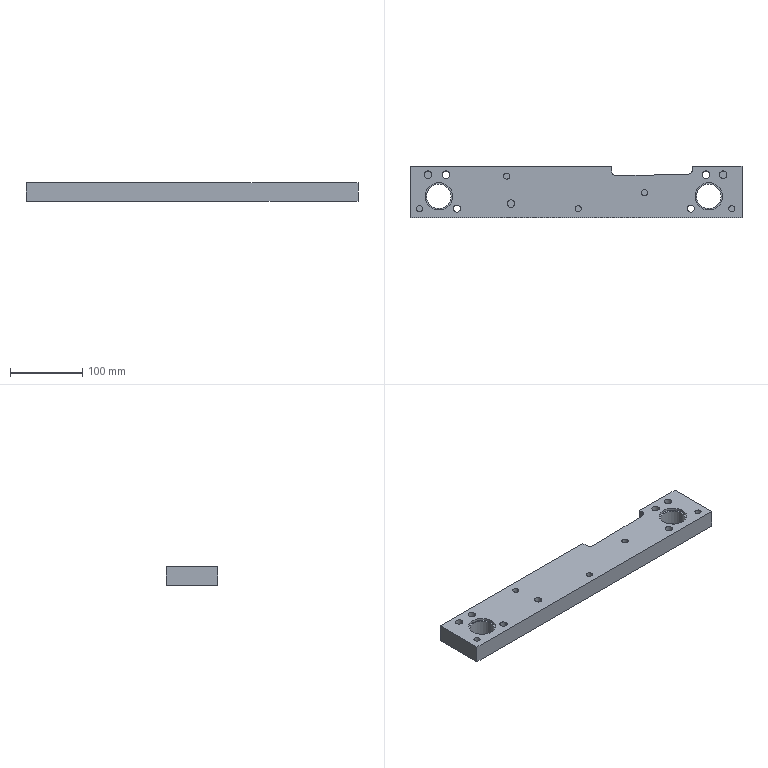Part | NX | features LIN_SOLID_COLOR 2 | 1 solid | 54 faces | box 460 x 72 x 25 mm | volume 695403 mm3 | plane 30 | cylinder 24 | commonest cylinder face diameters 8.5 x5 10.3 x5 10 x4 10.001 x2 10.31 x2 14 x2
STEP:
#1=CARTESIAN_POINT('',(747.152,-157.,0.));
#2=VERTEX_POINT('',#1);
#3=CARTESIAN_POINT('',(741.997,-157.,0.));
#4=DIRECTION('',(0.,0.,1.));
#5=DIRECTION('',(1.,0.,0.));
#6=AXIS2_PLACEMENT_3D('',#3,#4,#5);
#7=CIRCLE('',#6,5.155);
#8=EDGE_CURVE('',#2,#2,#7,.T.);
#9=ORIENTED_EDGE('',*,*,#8,.T.);
#10=EDGE_LOOP('',(#9));
#11=FACE_BOUND('',#10,.T.);
#12=CARTESIAN_POINT('',(423.158,-157.,0.));
#13=VERTEX_POINT('',#12);
#14=CARTESIAN_POINT('',(418.003,-157.,0.));
#15=DIRECTION('',(0.,0.,1.));
#16=DIRECTION('',(1.,0.,0.));
#17=AXIS2_PLACEMENT_3D('',#14,#15,#16);
#18=CIRCLE('',#17,5.155);
#19=EDGE_CURVE('',#13,#13,#18,.T.);
#20=ORIENTED_EDGE('',*,*,#19,.T.);
#21=EDGE_LOOP('',(#20));
#22=FACE_BOUND('',#21,.T.);
#23=CARTESIAN_POINT('',(750.,-140.,0.));
#24=VERTEX_POINT('',#23);
#25=CARTESIAN_POINT('',(767.,-140.,0.));
#26=DIRECTION('',(0.,0.,-1.));
#27=DIRECTION('',(-1.,0.,0.));
#28=AXIS2_PLACEMENT_3D('',#25,#26,#27);
#29=CIRCLE('',#28,17.);
#30=EDGE_CURVE('',#24,#24,#29,.T.);
#31=ORIENTED_EDGE('',*,*,#30,.F.);
#32=EDGE_LOOP('',(#31));
#33=FACE_BOUND('',#32,.T.);
#34=CARTESIAN_POINT('',(376.,-140.,0.));
#35=VERTEX_POINT('',#34);
#36=CARTESIAN_POINT('',(393.,-140.,0.));
#37=DIRECTION('',(0.,0.,-1.));
#38=DIRECTION('',(-1.,0.,0.));
#39=AXIS2_PLACEMENT_3D('',#36,#37,#38);
#40=CIRCLE('',#39,17.);
#41=EDGE_CURVE('',#35,#35,#40,.T.);
#42=ORIENTED_EDGE('',*,*,#41,.F.);
#43=EDGE_LOOP('',(#42));
#44=FACE_BOUND('',#43,.T.);
#45=CARTESIAN_POINT('',(757.85,-110.,0.));
#46=VERTEX_POINT('',#45);
#47=CARTESIAN_POINT('',(763.,-110.,0.));
#48=DIRECTION('',(0.,0.,-1.));
#49=DIRECTION('',(-1.,0.,0.));
#50=AXIS2_PLACEMENT_3D('',#47,#48,#49);
#51=CIRCLE('',#50,5.15);
#52=EDGE_CURVE('',#46,#46,#51,.T.);
#53=ORIENTED_EDGE('',*,*,#52,.F.);
#54=EDGE_LOOP('',(#53));
#55=FACE_BOUND('',#54,.T.);
#56=CARTESIAN_POINT('',(397.85,-110.,0.));
#57=VERTEX_POINT('',#56);
#58=CARTESIAN_POINT('',(403.,-110.,0.));
#59=DIRECTION('',(0.,0.,-1.));
#60=DIRECTION('',(-1.,0.,0.));
#61=AXIS2_PLACEMENT_3D('',#58,#59,#60);
#62=CIRCLE('',#61,5.15);
#63=EDGE_CURVE('',#57,#57,#62,.T.);
#64=ORIENTED_EDGE('',*,*,#63,.F.);
#65=EDGE_LOOP('',(#64));
#66=FACE_BOUND('',#65,.T.);
#67=CARTESIAN_POINT('',(646.028,-130.524,0.));
#68=VERTEX_POINT('',#67);
#69=CARTESIAN_POINT('',(638.826,-123.653,0.));
#70=VERTEX_POINT('',#69);
#71=CARTESIAN_POINT('',(642.098,-127.434,0.));
#72=DIRECTION('',(0.,0.,-1.));
#73=DIRECTION('',(-1.,0.,0.));
#74=AXIS2_PLACEMENT_3D('',#71,#72,#73);
#75=CIRCLE('',#74,5.);
#76=EDGE_CURVE('',#68,#70,#75,.T.);
#77=ORIENTED_EDGE('',*,*,#76,.F.);
#78=CARTESIAN_POINT('',(731.927,-128.503,0.));
#79=VERTEX_POINT('',#78);
#80=CARTESIAN_POINT('',(745.016,-128.195,0.));
#81=DIRECTION('',(-0.9997,-0.02352,0.));
#82=VECTOR('',#81,1000.);
#83=LINE('',#80,#82);
#84=EDGE_CURVE('',#79,#68,#83,.T.);
#85=ORIENTED_EDGE('',*,*,#84,.F.);
#86=CARTESIAN_POINT('',(738.798,-121.301,0.));
#87=VERTEX_POINT('',#86);
#88=CARTESIAN_POINT('',(735.708,-125.231,0.));
#89=DIRECTION('',(0.,0.,-1.));
#90=DIRECTION('',(-1.,0.,0.));
#91=AXIS2_PLACEMENT_3D('',#88,#89,#90);
#92=CIRCLE('',#91,5.);
#93=EDGE_CURVE('',#87,#79,#92,.T.);
#94=ORIENTED_EDGE('',*,*,#93,.F.);
#95=CARTESIAN_POINT('',(738.515,-109.271,0.));
#96=VERTEX_POINT('',#95);
#97=CARTESIAN_POINT('',(735.947,-0.1424,0.));
#98=DIRECTION('',(0.02352,-0.9997,0.));
#99=VECTOR('',#98,1000.);
#100=LINE('',#97,#99);
#101=EDGE_CURVE('',#96,#87,#100,.T.);
#102=ORIENTED_EDGE('',*,*,#101,.F.);
#103=CARTESIAN_POINT('',(744.35,-102.204,0.));
#104=VERTEX_POINT('',#103);
#105=CARTESIAN_POINT('',(737.352,-102.368,0.));
#106=DIRECTION('',(0.,0.,-1.));
#107=DIRECTION('',(-1.,0.,0.));
#108=AXIS2_PLACEMENT_3D('',#105,#106,#107);
#109=CIRCLE('',#108,7.);
#110=EDGE_CURVE('',#104,#96,#109,.T.);
#111=ORIENTED_EDGE('',*,*,#110,.F.);
#112=CARTESIAN_POINT('',(744.251,-98.,0.));
#113=VERTEX_POINT('',#112);
#114=CARTESIAN_POINT('',(741.946,-0.001282,0.));
#115=DIRECTION('',(-0.02352,0.9997,0.));
#116=VECTOR('',#115,1000.);
#117=LINE('',#114,#116);
#118=EDGE_CURVE('',#113,#104,#117,.F.);
#119=ORIENTED_EDGE('',*,*,#118,.F.);
#120=CARTESIAN_POINT('',(813.,-98.,0.));
#121=VERTEX_POINT('',#120);
#122=CARTESIAN_POINT('',(742.,-98.,0.));
#123=DIRECTION('',(1.,0.,0.));
#124=VECTOR('',#123,1000.);
#125=LINE('',#122,#124);
#126=EDGE_CURVE('',#113,#121,#125,.T.);
#127=ORIENTED_EDGE('',*,*,#126,.T.);
#128=CARTESIAN_POINT('',(813.,-170.,0.));
#129=VERTEX_POINT('',#128);
#130=CARTESIAN_POINT('',(813.,0.,0.));
#131=DIRECTION('',(0.,-1.,0.));
#132=VECTOR('',#131,1000.);
#133=LINE('',#130,#132);
#134=EDGE_CURVE('',#121,#129,#133,.T.);
#135=ORIENTED_EDGE('',*,*,#134,.T.);
#136=CARTESIAN_POINT('',(353.,-170.,0.));
#137=VERTEX_POINT('',#136);
#138=CARTESIAN_POINT('',(788.,-170.,0.));
#139=DIRECTION('',(1.,0.,0.));
#140=VECTOR('',#139,1000.);
#141=LINE('',#138,#140);
#142=EDGE_CURVE('',#137,#129,#141,.T.);
#143=ORIENTED_EDGE('',*,*,#142,.F.);
#144=CARTESIAN_POINT('',(353.,-98.,0.));
#145=VERTEX_POINT('',#144);
#146=CARTESIAN_POINT('',(353.,0.,0.));
#147=DIRECTION('',(0.,-1.,0.));
#148=VECTOR('',#147,1000.);
#149=LINE('',#146,#148);
#150=EDGE_CURVE('',#145,#137,#149,.T.);
#151=ORIENTED_EDGE('',*,*,#150,.F.);
#152=CARTESIAN_POINT('',(529.5,-98.,0.));
#153=VERTEX_POINT('',#152);
#154=CARTESIAN_POINT('',(742.,-98.,0.));
#155=DIRECTION('',(1.,0.,0.));
#156=VECTOR('',#155,1000.);
#157=LINE('',#154,#156);
#158=EDGE_CURVE('',#145,#153,#157,.T.);
#159=ORIENTED_EDGE('',*,*,#158,.T.);
#160=CARTESIAN_POINT('',(529.5,-111.161,0.));
#161=VERTEX_POINT('',#160);
#162=CARTESIAN_POINT('',(529.5,0.,0.));
#163=DIRECTION('',(0.,1.,0.));
#164=VECTOR('',#163,1000.);
#165=LINE('',#162,#164);
#166=EDGE_CURVE('',#161,#153,#165,.T.);
#167=ORIENTED_EDGE('',*,*,#166,.F.);
#168=CARTESIAN_POINT('',(536.539,-118.2,0.));
#169=VERTEX_POINT('',#168);
#170=CARTESIAN_POINT('',(532.682,-115.018,0.));
#171=DIRECTION('',(0.,0.,-1.));
#172=DIRECTION('',(-1.,0.,0.));
#173=AXIS2_PLACEMENT_3D('',#170,#171,#172);
#174=CIRCLE('',#173,5.);
#175=EDGE_CURVE('',#169,#161,#174,.T.);
#176=ORIENTED_EDGE('',*,*,#175,.F.);
#177=CARTESIAN_POINT('',(588.461,-118.2,0.));
#178=VERTEX_POINT('',#177);
#179=CARTESIAN_POINT('',(742.,-118.2,0.));
#180=DIRECTION('',(-1.,0.,0.));
#181=VECTOR('',#180,1000.);
#182=LINE('',#179,#181);
#183=EDGE_CURVE('',#178,#169,#182,.T.);
#184=ORIENTED_EDGE('',*,*,#183,.F.);
#185=CARTESIAN_POINT('',(595.5,-111.161,0.));
#186=VERTEX_POINT('',#185);
#187=CARTESIAN_POINT('',(592.318,-115.018,0.));
#188=DIRECTION('',(0.,0.,-1.));
#189=DIRECTION('',(-1.,0.,0.));
#190=AXIS2_PLACEMENT_3D('',#187,#188,#189);
#191=CIRCLE('',#190,5.);
#192=EDGE_CURVE('',#186,#178,#191,.T.);
#193=ORIENTED_EDGE('',*,*,#192,.F.);
#194=CARTESIAN_POINT('',(595.5,-98.,0.));
#195=VERTEX_POINT('',#194);
#196=CARTESIAN_POINT('',(595.5,0.,0.));
#197=DIRECTION('',(0.,-1.,0.));
#198=VECTOR('',#197,1000.);
#199=LINE('',#196,#198);
#200=EDGE_CURVE('',#195,#186,#199,.T.);
#201=ORIENTED_EDGE('',*,*,#200,.F.);
#202=CARTESIAN_POINT('',(632.22,-98.,0.));
#203=VERTEX_POINT('',#202);
#204=CARTESIAN_POINT('',(742.,-98.,0.));
#205=DIRECTION('',(1.,0.,0.));
#206=VECTOR('',#205,1000.);
#207=LINE('',#204,#206);
#208=EDGE_CURVE('',#195,#203,#207,.T.);
#209=ORIENTED_EDGE('',*,*,#208,.T.);
#210=CARTESIAN_POINT('',(632.381,-104.838,0.));
#211=VERTEX_POINT('',#210);
#212=CARTESIAN_POINT('',(629.977,-2.636,0.));
#213=DIRECTION('',(-0.02352,0.9997,0.));
#214=VECTOR('',#213,1000.);
#215=LINE('',#212,#214);
#216=EDGE_CURVE('',#211,#203,#215,.T.);
#217=ORIENTED_EDGE('',*,*,#216,.F.);
#218=CARTESIAN_POINT('',(638.543,-111.623,0.));
#219=VERTEX_POINT('',#218);
#220=CARTESIAN_POINT('',(639.379,-104.674,0.));
#221=DIRECTION('',(0.,0.,-1.));
#222=DIRECTION('',(-1.,0.,0.));
#223=AXIS2_PLACEMENT_3D('',#220,#221,#222);
#224=CIRCLE('',#223,7.);
#225=EDGE_CURVE('',#219,#211,#224,.T.);
#226=ORIENTED_EDGE('',*,*,#225,.F.);
#227=CARTESIAN_POINT('',(635.975,-2.495,0.));
#228=DIRECTION('',(-0.02352,0.9997,0.));
#229=VECTOR('',#228,1000.);
#230=LINE('',#227,#229);
#231=EDGE_CURVE('',#70,#219,#230,.T.);
#232=ORIENTED_EDGE('',*,*,#231,.F.);
#233=EDGE_LOOP('',(#77,#85,#94,#102,#111,#119,#127,#135,#143,#151,#159,#167,#176,#184,#193,#201,#209,#217,#226,#232));
#234=FACE_BOUND('',#233,.T.);
#235=CARTESIAN_POINT('',(742.,0.,0.));
#236=DIRECTION('',(0.,0.,-1.));
#237=DIRECTION('',(-1.,0.,0.));
#238=AXIS2_PLACEMENT_3D('',#235,#236,#237);
#239=PLANE('',#238);
#240=ADVANCED_FACE('',(#11,#22,#33,#44,#55,#66,#234),#239,.T.);
#241=CARTESIAN_POINT('',(590.25,-157.,1.));
#242=VERTEX_POINT('',#241);
#243=CARTESIAN_POINT('',(586.,-157.,1.));
#244=DIRECTION('',(0.,0.,1.));
#245=DIRECTION('',(1.,0.,0.));
#246=AXIS2_PLACEMENT_3D('',#243,#244,#245);
#247=CIRCLE('',#246,4.25);
#248=EDGE_CURVE('',#242,#242,#247,.F.);
#249=ORIENTED_EDGE('',*,*,#248,.T.);
#250=EDGE_LOOP('',(#249));
#251=FACE_BOUND('',#250,.T.);
#252=CARTESIAN_POINT('',(590.25,-157.,25.));
#253=VERTEX_POINT('',#252);
#254=CARTESIAN_POINT('',(586.,-157.,25.));
#255=DIRECTION('',(0.,0.,1.));
#256=DIRECTION('',(1.,0.,0.));
#257=AXIS2_PLACEMENT_3D('',#254,#255,#256);
#258=CIRCLE('',#257,4.25);
#259=EDGE_CURVE('',#253,#253,#258,.T.);
#260=ORIENTED_EDGE('',*,*,#259,.T.);
#261=EDGE_LOOP('',(#260));
#262=FACE_BOUND('',#261,.T.);
#263=CARTESIAN_POINT('',(586.,-157.,25.1));
#264=DIRECTION('',(0.,0.,-1.));
#265=DIRECTION('',(1.,0.,0.));
#266=AXIS2_PLACEMENT_3D('',#263,#264,#265);
#267=CYLINDRICAL_SURFACE('',#266,4.25);
#268=ADVANCED_FACE('',(#251,#262),#267,.F.);
#269=CARTESIAN_POINT('',(410.,-140.,21.7));
#270=VERTEX_POINT('',#269);
#271=CARTESIAN_POINT('',(393.,-140.,21.7));
#272=DIRECTION('',(0.,0.,1.));
#273=DIRECTION('',(1.,0.,0.));
#274=AXIS2_PLACEMENT_3D('',#271,#272,#273);
#275=CIRCLE('',#274,17.);
#276=EDGE_CURVE('',#270,#270,#275,.F.);
#277=ORIENTED_EDGE('',*,*,#276,.T.);
#278=EDGE_LOOP('',(#277));
#279=FACE_BOUND('',#278,.T.);
#280=CARTESIAN_POINT('',(412.,-140.,21.7));
#281=VERTEX_POINT('',#280);
#282=CARTESIAN_POINT('',(393.,-140.,21.7));
#283=DIRECTION('',(0.,0.,1.));
#284=DIRECTION('',(1.,0.,0.));
#285=AXIS2_PLACEMENT_3D('',#282,#283,#284);
#286=CIRCLE('',#285,19.);
#287=EDGE_CURVE('',#281,#281,#286,.F.);
#288=ORIENTED_EDGE('',*,*,#287,.F.);
#289=EDGE_LOOP('',(#288));
#290=FACE_BOUND('',#289,.T.);
#291=CARTESIAN_POINT('',(393.,-140.,21.7));
#292=DIRECTION('',(0.,0.,1.));
#293=DIRECTION('',(1.,0.,0.));
#294=AXIS2_PLACEMENT_3D('',#291,#292,#293);
#295=PLANE('',#294);
#296=ADVANCED_FACE('',(#279,#290),#295,.T.);
#297=CARTESIAN_POINT('',(784.,-140.,21.7));
#298=VERTEX_POINT('',#297);
#299=CARTESIAN_POINT('',(767.,-140.,21.7));
#300=DIRECTION('',(0.,0.,1.));
#301=DIRECTION('',(1.,0.,0.));
#302=AXIS2_PLACEMENT_3D('',#299,#300,#301);
#303=CIRCLE('',#302,17.);
#304=EDGE_CURVE('',#298,#298,#303,.F.);
#305=ORIENTED_EDGE('',*,*,#304,.T.);
#306=EDGE_LOOP('',(#305));
#307=FACE_BOUND('',#306,.T.);
#308=CARTESIAN_POINT('',(786.,-140.,21.7));
#309=VERTEX_POINT('',#308);
#310=CARTESIAN_POINT('',(767.,-140.,21.7));
#311=DIRECTION('',(0.,0.,1.));
#312=DIRECTION('',(1.,0.,0.));
#313=AXIS2_PLACEMENT_3D('',#310,#311,#312);
#314=CIRCLE('',#313,19.);
#315=EDGE_CURVE('',#309,#309,#314,.F.);
#316=ORIENTED_EDGE('',*,*,#315,.F.);
#317=EDGE_LOOP('',(#316));
#318=FACE_BOUND('',#317,.T.);
#319=CARTESIAN_POINT('',(767.,-140.,21.7));
#320=DIRECTION('',(0.,0.,1.));
#321=DIRECTION('',(1.,0.,0.));
#322=AXIS2_PLACEMENT_3D('',#319,#320,#321);
#323=PLANE('',#322);
#324=ADVANCED_FACE('',(#307,#318),#323,.T.);
#325=CARTESIAN_POINT('',(595.5,-111.161,13.5));
#326=VERTEX_POINT('',#325);
#327=CARTESIAN_POINT('',(588.461,-118.2,13.5));
#328=VERTEX_POINT('',#327);
#329=CARTESIAN_POINT('',(592.318,-115.018,13.5));
#330=DIRECTION('',(0.,0.,-1.));
#331=DIRECTION('',(1.,0.,0.));
#332=AXIS2_PLACEMENT_3D('',#329,#330,#331);
#333=CIRCLE('',#332,5.);
#334=EDGE_CURVE('',#326,#328,#333,.T.);
#335=ORIENTED_EDGE('',*,*,#334,.T.);
#336=CARTESIAN_POINT('',(536.539,-118.2,13.5));
#337=VERTEX_POINT('',#336);
#338=CARTESIAN_POINT('',(572.,-118.2,13.5));
#339=DIRECTION('',(-1.,0.,0.));
#340=VECTOR('',#339,1000.);
#341=LINE('',#338,#340);
#342=EDGE_CURVE('',#328,#337,#341,.T.);
#343=ORIENTED_EDGE('',*,*,#342,.T.);
#344=CARTESIAN_POINT('',(529.5,-111.161,13.5));
#345=VERTEX_POINT('',#344);
#346=CARTESIAN_POINT('',(532.682,-115.018,13.5));
#347=DIRECTION('',(0.,0.,-1.));
#348=DIRECTION('',(1.,0.,0.));
#349=AXIS2_PLACEMENT_3D('',#346,#347,#348);
#350=CIRCLE('',#349,5.);
#351=EDGE_CURVE('',#337,#345,#350,.T.);
#352=ORIENTED_EDGE('',*,*,#351,.T.);
#353=CARTESIAN_POINT('',(529.5,-98.,13.5));
#354=VERTEX_POINT('',#353);
#355=CARTESIAN_POINT('',(529.5,-110.2,13.5));
#356=DIRECTION('',(0.,1.,0.));
#357=VECTOR('',#356,1000.);
#358=LINE('',#355,#357);
#359=EDGE_CURVE('',#345,#354,#358,.T.);
#360=ORIENTED_EDGE('',*,*,#359,.T.);
#361=CARTESIAN_POINT('',(595.5,-98.,13.5));
#362=VERTEX_POINT('',#361);
#363=CARTESIAN_POINT('',(562.,-98.,13.5));
#364=DIRECTION('',(1.,0.,0.));
#365=VECTOR('',#364,1000.);
#366=LINE('',#363,#365);
#367=EDGE_CURVE('',#354,#362,#366,.T.);
#368=ORIENTED_EDGE('',*,*,#367,.T.);
#369=CARTESIAN_POINT('',(595.5,-90.2,13.5));
#370=DIRECTION('',(0.,-1.,0.));
#371=VECTOR('',#370,1000.);
#372=LINE('',#369,#371);
#373=EDGE_CURVE('',#362,#326,#372,.T.);
#374=ORIENTED_EDGE('',*,*,#373,.T.);
#375=EDGE_LOOP('',(#335,#343,#352,#360,#368,#374));
#376=FACE_BOUND('',#375,.T.);
#377=CARTESIAN_POINT('',(552.555,-107.951,13.5));
#378=DIRECTION('',(0.,0.,1.));
#379=DIRECTION('',(1.,0.,0.));
#380=AXIS2_PLACEMENT_3D('',#377,#378,#379);
#381=PLANE('',#380);
#382=ADVANCED_FACE('',(#376),#381,.F.);
#383=CARTESIAN_POINT('',(786.,-140.,25.));
#384=VERTEX_POINT('',#383);
#385=CARTESIAN_POINT('',(767.,-140.,25.));
#386=DIRECTION('',(0.,0.,1.));
#387=DIRECTION('',(1.,0.,0.));
#388=AXIS2_PLACEMENT_3D('',#385,#386,#387);
#389=CIRCLE('',#388,19.);
#390=EDGE_CURVE('',#384,#384,#389,.T.);
#391=ORIENTED_EDGE('',*,*,#390,.T.);
#392=EDGE_LOOP('',(#391));
#393=FACE_BOUND('',#392,.T.);
#394=ORIENTED_EDGE('',*,*,#315,.T.);
#395=EDGE_LOOP('',(#394));
#396=FACE_BOUND('',#395,.T.);
#397=CARTESIAN_POINT('',(767.,-140.,21.5));
#398=DIRECTION('',(0.,0.,1.));
#399=DIRECTION('',(1.,0.,0.));
#400=AXIS2_PLACEMENT_3D('',#397,#398,#399);
#401=CYLINDRICAL_SURFACE('',#400,19.);
#402=ADVANCED_FACE('',(#393,#396),#401,.F.);
#403=CARTESIAN_POINT('',(412.,-140.,25.));
#404=VERTEX_POINT('',#403);
#405=CARTESIAN_POINT('',(393.,-140.,25.));
#406=DIRECTION('',(0.,0.,1.));
#407=DIRECTION('',(1.,0.,0.));
#408=AXIS2_PLACEMENT_3D('',#405,#406,#407);
#409=CIRCLE('',#408,19.);
#410=EDGE_CURVE('',#404,#404,#409,.T.);
#411=ORIENTED_EDGE('',*,*,#410,.T.);
#412=EDGE_LOOP('',(#411));
#413=FACE_BOUND('',#412,.T.);
#414=ORIENTED_EDGE('',*,*,#287,.T.);
#415=EDGE_LOOP('',(#414));
#416=FACE_BOUND('',#415,.T.);
#417=CARTESIAN_POINT('',(393.,-140.,21.5));
#418=DIRECTION('',(0.,0.,1.));
#419=DIRECTION('',(1.,0.,0.));
#420=AXIS2_PLACEMENT_3D('',#417,#418,#419);
#421=CYLINDRICAL_SURFACE('',#420,19.);
#422=ADVANCED_FACE('',(#413,#416),#421,.F.);
#423=ORIENTED_EDGE('',*,*,#41,.T.);
#424=EDGE_LOOP('',(#423));
#425=FACE_BOUND('',#424,.T.);
#426=ORIENTED_EDGE('',*,*,#276,.F.);
#427=EDGE_LOOP('',(#426));
#428=FACE_BOUND('',#427,.T.);
#429=CARTESIAN_POINT('',(393.,-140.,36.));
#430=DIRECTION('',(0.,0.,-1.));
#431=DIRECTION('',(-1.,0.,0.));
#432=AXIS2_PLACEMENT_3D('',#429,#430,#431);
#433=CYLINDRICAL_SURFACE('',#432,17.);
#434=ADVANCED_FACE('',(#425,#428),#433,.F.);
#435=ORIENTED_EDGE('',*,*,#30,.T.);
#436=EDGE_LOOP('',(#435));
#437=FACE_BOUND('',#436,.T.);
#438=ORIENTED_EDGE('',*,*,#304,.F.);
#439=EDGE_LOOP('',(#438));
#440=FACE_BOUND('',#439,.T.);
#441=CARTESIAN_POINT('',(767.,-140.,36.));
#442=DIRECTION('',(0.,0.,-1.));
#443=DIRECTION('',(-1.,0.,0.));
#444=AXIS2_PLACEMENT_3D('',#441,#442,#443);
#445=CYLINDRICAL_SURFACE('',#444,17.);
#446=ADVANCED_FACE('',(#437,#440),#445,.F.);
#447=CARTESIAN_POINT('',(491.25,-112.,1.));
#448=VERTEX_POINT('',#447);
#449=CARTESIAN_POINT('',(487.,-112.,1.));
#450=DIRECTION('',(0.,0.,1.));
#451=DIRECTION('',(1.,0.,0.));
#452=AXIS2_PLACEMENT_3D('',#449,#450,#451);
#453=CIRCLE('',#452,4.25);
#454=EDGE_CURVE('',#448,#448,#453,.F.);
#455=ORIENTED_EDGE('',*,*,#454,.T.);
#456=EDGE_LOOP('',(#455));
#457=FACE_BOUND('',#456,.T.);
#458=CARTESIAN_POINT('',(491.25,-112.,25.));
#459=VERTEX_POINT('',#458);
#460=CARTESIAN_POINT('',(487.,-112.,25.));
#461=DIRECTION('',(0.,0.,1.));
#462=DIRECTION('',(1.,0.,0.));
#463=AXIS2_PLACEMENT_3D('',#460,#461,#462);
#464=CIRCLE('',#463,4.25);
#465=EDGE_CURVE('',#459,#459,#464,.T.);
#466=ORIENTED_EDGE('',*,*,#465,.T.);
#467=EDGE_LOOP('',(#466));
#468=FACE_BOUND('',#467,.T.);
#469=CARTESIAN_POINT('',(487.,-112.,25.1));
#470=DIRECTION('',(0.,0.,-1.));
#471=DIRECTION('',(1.,0.,0.));
#472=AXIS2_PLACEMENT_3D('',#469,#470,#471);
#473=CYLINDRICAL_SURFACE('',#472,4.25);
#474=ADVANCED_FACE('',(#457,#468),#473,.F.);
#475=CARTESIAN_POINT('',(370.25,-157.,1.));
#476=VERTEX_POINT('',#475);
#477=CARTESIAN_POINT('',(366.,-157.,1.));
#478=DIRECTION('',(0.,0.,1.));
#479=DIRECTION('',(1.,0.,0.));
#480=AXIS2_PLACEMENT_3D('',#477,#478,#479);
#481=CIRCLE('',#480,4.25);
#482=EDGE_CURVE('',#476,#476,#481,.F.);
#483=ORIENTED_EDGE('',*,*,#482,.T.);
#484=EDGE_LOOP('',(#483));
#485=FACE_BOUND('',#484,.T.);
#486=CARTESIAN_POINT('',(370.25,-157.,25.));
#487=VERTEX_POINT('',#486);
#488=CARTESIAN_POINT('',(366.,-157.,25.));
#489=DIRECTION('',(0.,0.,1.));
#490=DIRECTION('',(1.,0.,0.));
#491=AXIS2_PLACEMENT_3D('',#488,#489,#490);
#492=CIRCLE('',#491,4.25);
#493=EDGE_CURVE('',#487,#487,#492,.T.);
#494=ORIENTED_EDGE('',*,*,#493,.T.);
#495=EDGE_LOOP('',(#494));
#496=FACE_BOUND('',#495,.T.);
#497=CARTESIAN_POINT('',(366.,-157.,25.1));
#498=DIRECTION('',(0.,0.,-1.));
#499=DIRECTION('',(1.,0.,0.));
#500=AXIS2_PLACEMENT_3D('',#497,#498,#499);
#501=CYLINDRICAL_SURFACE('',#500,4.25);
#502=ADVANCED_FACE('',(#485,#496),#501,.F.);
#503=CARTESIAN_POINT('',(803.25,-157.,1.));
#504=VERTEX_POINT('',#503);
#505=CARTESIAN_POINT('',(799.,-157.,1.));
#506=DIRECTION('',(0.,0.,1.));
#507=DIRECTION('',(1.,0.,0.));
#508=AXIS2_PLACEMENT_3D('',#505,#506,#507);
#509=CIRCLE('',#508,4.25);
#510=EDGE_CURVE('',#504,#504,#509,.F.);
#511=ORIENTED_EDGE('',*,*,#510,.T.);
#512=EDGE_LOOP('',(#511));
#513=FACE_BOUND('',#512,.T.);
#514=CARTESIAN_POINT('',(803.25,-157.,25.));
#515=VERTEX_POINT('',#514);
#516=CARTESIAN_POINT('',(799.,-157.,25.));
#517=DIRECTION('',(0.,0.,1.));
#518=DIRECTION('',(1.,0.,0.));
#519=AXIS2_PLACEMENT_3D('',#516,#517,#518);
#520=CIRCLE('',#519,4.25);
#521=EDGE_CURVE('',#515,#515,#520,.T.);
#522=ORIENTED_EDGE('',*,*,#521,.T.);
#523=EDGE_LOOP('',(#522));
#524=FACE_BOUND('',#523,.T.);
#525=CARTESIAN_POINT('',(799.,-157.,25.1));
#526=DIRECTION('',(0.,0.,-1.));
#527=DIRECTION('',(1.,0.,0.));
#528=AXIS2_PLACEMENT_3D('',#525,#526,#527);
#529=CYLINDRICAL_SURFACE('',#528,4.25);
#530=ADVANCED_FACE('',(#513,#524),#529,.F.);
#531=CARTESIAN_POINT('',(423.004,-157.,12.));
#532=VERTEX_POINT('',#531);
#533=CARTESIAN_POINT('',(418.003,-157.,12.));
#534=DIRECTION('',(0.,0.,1.));
#535=DIRECTION('',(1.,0.,0.));
#536=AXIS2_PLACEMENT_3D('',#533,#534,#535);
#537=CIRCLE('',#536,5.);
#538=EDGE_CURVE('',#532,#532,#537,.F.);
#539=ORIENTED_EDGE('',*,*,#538,.T.);
#540=EDGE_LOOP('',(#539));
#541=FACE_BOUND('',#540,.T.);
#542=CARTESIAN_POINT('',(423.004,-157.,25.));
#543=VERTEX_POINT('',#542);
#544=CARTESIAN_POINT('',(418.003,-157.,25.));
#545=DIRECTION('',(0.,0.,1.));
#546=DIRECTION('',(1.,0.,0.));
#547=AXIS2_PLACEMENT_3D('',#544,#545,#546);
#548=CIRCLE('',#547,5.);
#549=EDGE_CURVE('',#543,#543,#548,.T.);
#550=ORIENTED_EDGE('',*,*,#549,.T.);
#551=EDGE_LOOP('',(#550));
#552=FACE_BOUND('',#551,.T.);
#553=CARTESIAN_POINT('',(418.003,-157.,25.1));
#554=DIRECTION('',(0.,0.,-1.));
#555=DIRECTION('',(1.,0.,0.));
#556=AXIS2_PLACEMENT_3D('',#553,#554,#555);
#557=CYLINDRICAL_SURFACE('',#556,5.);
#558=ADVANCED_FACE('',(#541,#552),#557,.F.);
#559=CARTESIAN_POINT('',(746.997,-157.,12.));
#560=VERTEX_POINT('',#559);
#561=CARTESIAN_POINT('',(741.997,-157.,12.));
#562=DIRECTION('',(0.,0.,1.));
#563=DIRECTION('',(1.,0.,0.));
#564=AXIS2_PLACEMENT_3D('',#561,#562,#563);
#565=CIRCLE('',#564,5.);
#566=EDGE_CURVE('',#560,#560,#565,.F.);
#567=ORIENTED_EDGE('',*,*,#566,.T.);
#568=EDGE_LOOP('',(#567));
#569=FACE_BOUND('',#568,.T.);
#570=CARTESIAN_POINT('',(746.997,-157.,25.));
#571=VERTEX_POINT('',#570);
#572=CARTESIAN_POINT('',(741.997,-157.,25.));
#573=DIRECTION('',(0.,0.,1.));
#574=DIRECTION('',(1.,0.,0.));
#575=AXIS2_PLACEMENT_3D('',#572,#573,#574);
#576=CIRCLE('',#575,5.);
#577=EDGE_CURVE('',#571,#571,#576,.T.);
#578=ORIENTED_EDGE('',*,*,#577,.T.);
#579=EDGE_LOOP('',(#578));
#580=FACE_BOUND('',#579,.T.);
#581=CARTESIAN_POINT('',(741.997,-157.,25.1));
#582=DIRECTION('',(0.,0.,-1.));
#583=DIRECTION('',(1.,0.,0.));
#584=AXIS2_PLACEMENT_3D('',#581,#582,#583);
#585=CYLINDRICAL_SURFACE('',#584,5.);
#586=ADVANCED_FACE('',(#569,#580),#585,.F.);
#587=CARTESIAN_POINT('',(383.15,-110.,1.));
#588=VERTEX_POINT('',#587);
#589=CARTESIAN_POINT('',(378.,-110.,1.));
#590=DIRECTION('',(0.,0.,1.));
#591=DIRECTION('',(1.,0.,0.));
#592=AXIS2_PLACEMENT_3D('',#589,#590,#591);
#593=CIRCLE('',#592,5.15);
#594=EDGE_CURVE('',#588,#588,#593,.F.);
#595=ORIENTED_EDGE('',*,*,#594,.T.);
#596=EDGE_LOOP('',(#595));
#597=FACE_BOUND('',#596,.T.);
#598=CARTESIAN_POINT('',(383.15,-110.,25.));
#599=VERTEX_POINT('',#598);
#600=CARTESIAN_POINT('',(378.,-110.,25.));
#601=DIRECTION('',(0.,0.,1.));
#602=DIRECTION('',(1.,0.,0.));
#603=AXIS2_PLACEMENT_3D('',#600,#601,#602);
#604=CIRCLE('',#603,5.15);
#605=EDGE_CURVE('',#599,#599,#604,.F.);
#606=ORIENTED_EDGE('',*,*,#605,.F.);
#607=EDGE_LOOP('',(#606));
#608=FACE_BOUND('',#607,.T.);
#609=CARTESIAN_POINT('',(378.,-110.,25.));
#610=DIRECTION('',(0.,0.,-1.));
#611=DIRECTION('',(1.,0.,0.));
#612=AXIS2_PLACEMENT_3D('',#609,#610,#611);
#613=CYLINDRICAL_SURFACE('',#612,5.15);
#614=ADVANCED_FACE('',(#597,#608),#613,.F.);
#615=CARTESIAN_POINT('',(792.15,-110.,1.));
#616=VERTEX_POINT('',#615);
#617=CARTESIAN_POINT('',(787.,-110.,1.));
#618=DIRECTION('',(0.,0.,1.));
#619=DIRECTION('',(1.,0.,0.));
#620=AXIS2_PLACEMENT_3D('',#617,#618,#619);
#621=CIRCLE('',#620,5.15);
#622=EDGE_CURVE('',#616,#616,#621,.F.);
#623=ORIENTED_EDGE('',*,*,#622,.T.);
#624=EDGE_LOOP('',(#623));
#625=FACE_BOUND('',#624,.T.);
#626=CARTESIAN_POINT('',(792.15,-110.,25.));
#627=VERTEX_POINT('',#626);
#628=CARTESIAN_POINT('',(787.,-110.,25.));
#629=DIRECTION('',(0.,0.,1.));
#630=DIRECTION('',(1.,0.,0.));
#631=AXIS2_PLACEMENT_3D('',#628,#629,#630);
#632=CIRCLE('',#631,5.15);
#633=EDGE_CURVE('',#627,#627,#632,.F.);
#634=ORIENTED_EDGE('',*,*,#633,.F.);
#635=EDGE_LOOP('',(#634));
#636=FACE_BOUND('',#635,.T.);
#637=CARTESIAN_POINT('',(787.,-110.,25.));
#638=DIRECTION('',(0.,0.,-1.));
#639=DIRECTION('',(1.,0.,0.));
#640=AXIS2_PLACEMENT_3D('',#637,#638,#639);
#641=CYLINDRICAL_SURFACE('',#640,5.15);
#642=ADVANCED_FACE('',(#625,#636),#641,.F.);
#643=CARTESIAN_POINT('',(498.15,-150.,1.));
#644=VERTEX_POINT('',#643);
#645=CARTESIAN_POINT('',(493.,-150.,1.));
#646=DIRECTION('',(0.,0.,1.));
#647=DIRECTION('',(1.,0.,0.));
#648=AXIS2_PLACEMENT_3D('',#645,#646,#647);
#649=CIRCLE('',#648,5.15);
#650=EDGE_CURVE('',#644,#644,#649,.F.);
#651=ORIENTED_EDGE('',*,*,#650,.T.);
#652=EDGE_LOOP('',(#651));
#653=FACE_BOUND('',#652,.T.);
#654=CARTESIAN_POINT('',(498.15,-150.,25.));
#655=VERTEX_POINT('',#654);
#656=CARTESIAN_POINT('',(493.,-150.,25.));
#657=DIRECTION('',(0.,0.,1.));
#658=DIRECTION('',(1.,0.,0.));
#659=AXIS2_PLACEMENT_3D('',#656,#657,#658);
#660=CIRCLE('',#659,5.15);
#661=EDGE_CURVE('',#655,#655,#660,.F.);
#662=ORIENTED_EDGE('',*,*,#661,.F.);
#663=EDGE_LOOP('',(#662));
#664=FACE_BOUND('',#663,.T.);
#665=CARTESIAN_POINT('',(493.,-150.,25.));
#666=DIRECTION('',(0.,0.,-1.));
#667=DIRECTION('',(1.,0.,0.));
#668=AXIS2_PLACEMENT_3D('',#665,#666,#667);
#669=CYLINDRICAL_SURFACE('',#668,5.15);
#670=ADVANCED_FACE('',(#653,#664),#669,.F.);
#671=ORIENTED_EDGE('',*,*,#342,.F.);
#672=CARTESIAN_POINT('',(588.461,-118.2,13.5));
#673=DIRECTION('',(0.,0.,-1.));
#674=VECTOR('',#673,1000.);
#675=LINE('',#672,#674);
#676=EDGE_CURVE('',#328,#178,#675,.T.);
#677=ORIENTED_EDGE('',*,*,#676,.T.);
#678=ORIENTED_EDGE('',*,*,#183,.T.);
#679=CARTESIAN_POINT('',(536.539,-118.2,13.5));
#680=DIRECTION('',(0.,0.,-1.));
#681=VECTOR('',#680,1000.);
#682=LINE('',#679,#681);
#683=EDGE_CURVE('',#169,#337,#682,.F.);
#684=ORIENTED_EDGE('',*,*,#683,.T.);
#685=EDGE_LOOP('',(#671,#677,#678,#684));
#686=FACE_BOUND('',#685,.T.);
#687=CARTESIAN_POINT('',(572.,-118.2,-36.501));
#688=DIRECTION('',(0.,-1.,0.));
#689=DIRECTION('',(0.,0.,-1.));
#690=AXIS2_PLACEMENT_3D('',#687,#688,#689);
#691=PLANE('',#690);
#692=ADVANCED_FACE('',(#686),#691,.F.);
#693=ORIENTED_EDGE('',*,*,#175,.T.);
#694=CARTESIAN_POINT('',(529.5,-111.161,13.5));
#695=DIRECTION('',(0.,0.,-1.));
#696=VECTOR('',#695,1000.);
#697=LINE('',#694,#696);
#698=EDGE_CURVE('',#345,#161,#697,.T.);
#699=ORIENTED_EDGE('',*,*,#698,.F.);
#700=ORIENTED_EDGE('',*,*,#351,.F.);
#701=ORIENTED_EDGE('',*,*,#683,.F.);
#702=EDGE_LOOP('',(#693,#699,#700,#701));
#703=FACE_BOUND('',#702,.T.);
#704=CARTESIAN_POINT('',(532.682,-115.018,13.5));
#705=DIRECTION('',(0.,0.,-1.));
#706=DIRECTION('',(1.,0.,0.));
#707=AXIS2_PLACEMENT_3D('',#704,#705,#706);
#708=CYLINDRICAL_SURFACE('',#707,5.);
#709=ADVANCED_FACE('',(#703),#708,.F.);
#710=ORIENTED_EDGE('',*,*,#359,.F.);
#711=ORIENTED_EDGE('',*,*,#698,.T.);
#712=ORIENTED_EDGE('',*,*,#166,.T.);
#713=CARTESIAN_POINT('',(529.5,-98.,12.5));
#714=DIRECTION('',(0.,0.,1.));
#715=VECTOR('',#714,1000.);
#716=LINE('',#713,#715);
#717=EDGE_CURVE('',#153,#354,#716,.T.);
#718=ORIENTED_EDGE('',*,*,#717,.T.);
#719=EDGE_LOOP('',(#710,#711,#712,#718));
#720=FACE_BOUND('',#719,.T.);
#721=CARTESIAN_POINT('',(529.5,-110.2,-36.501));
#722=DIRECTION('',(-1.,0.,0.));
#723=DIRECTION('',(0.,0.,1.));
#724=AXIS2_PLACEMENT_3D('',#721,#722,#723);
#725=PLANE('',#724);
#726=ADVANCED_FACE('',(#720),#725,.F.);
#727=CARTESIAN_POINT('',(353.,-170.,25.));
#728=VERTEX_POINT('',#727);
#729=CARTESIAN_POINT('',(353.,-98.,25.));
#730=VERTEX_POINT('',#729);
#731=CARTESIAN_POINT('',(353.,0.,25.));
#732=DIRECTION('',(0.,1.,0.));
#733=VECTOR('',#732,1000.);
#734=LINE('',#731,#733);
#735=EDGE_CURVE('',#728,#730,#734,.T.);
#736=ORIENTED_EDGE('',*,*,#735,.T.);
#737=CARTESIAN_POINT('',(353.,-98.,25.));
#738=DIRECTION('',(0.,0.,-1.));
#739=VECTOR('',#738,1000.);
#740=LINE('',#737,#739);
#741=EDGE_CURVE('',#730,#145,#740,.T.);
#742=ORIENTED_EDGE('',*,*,#741,.T.);
#743=ORIENTED_EDGE('',*,*,#150,.T.);
#744=CARTESIAN_POINT('',(353.,-170.,25.));
#745=DIRECTION('',(0.,0.,1.));
#746=VECTOR('',#745,1000.);
#747=LINE('',#744,#746);
#748=EDGE_CURVE('',#137,#728,#747,.T.);
#749=ORIENTED_EDGE('',*,*,#748,.T.);
#750=EDGE_LOOP('',(#736,#742,#743,#749));
#751=FACE_BOUND('',#750,.T.);
#752=CARTESIAN_POINT('',(353.,0.,25.));
#753=DIRECTION('',(-1.,0.,0.));
#754=DIRECTION('',(0.,0.,1.));
#755=AXIS2_PLACEMENT_3D('',#752,#753,#754);
#756=PLANE('',#755);
#757=ADVANCED_FACE('',(#751),#756,.T.);
#758=ORIENTED_EDGE('',*,*,#142,.T.);
#759=CARTESIAN_POINT('',(813.,-170.,25.));
#760=VERTEX_POINT('',#759);
#761=CARTESIAN_POINT('',(813.,-170.,25.));
#762=DIRECTION('',(0.,0.,1.));
#763=VECTOR('',#762,1000.);
#764=LINE('',#761,#763);
#765=EDGE_CURVE('',#129,#760,#764,.T.);
#766=ORIENTED_EDGE('',*,*,#765,.T.);
#767=CARTESIAN_POINT('',(788.,-170.,25.));
#768=DIRECTION('',(-1.,0.,0.));
#769=VECTOR('',#768,1000.);
#770=LINE('',#767,#769);
#771=EDGE_CURVE('',#760,#728,#770,.T.);
#772=ORIENTED_EDGE('',*,*,#771,.T.);
#773=ORIENTED_EDGE('',*,*,#748,.F.);
#774=EDGE_LOOP('',(#758,#766,#772,#773));
#775=FACE_BOUND('',#774,.T.);
#776=CARTESIAN_POINT('',(788.,-170.,25.));
#777=DIRECTION('',(0.,-1.,0.));
#778=DIRECTION('',(0.,0.,-1.));
#779=AXIS2_PLACEMENT_3D('',#776,#777,#778);
#780=PLANE('',#779);
#781=ADVANCED_FACE('',(#775),#780,.T.);
#782=ORIENTED_EDGE('',*,*,#134,.F.);
#783=CARTESIAN_POINT('',(813.,-98.,25.));
#784=VERTEX_POINT('',#783);
#785=CARTESIAN_POINT('',(813.,-98.,12.5));
#786=DIRECTION('',(0.,0.,1.));
#787=VECTOR('',#786,1000.);
#788=LINE('',#785,#787);
#789=EDGE_CURVE('',#121,#784,#788,.T.);
#790=ORIENTED_EDGE('',*,*,#789,.T.);
#791=CARTESIAN_POINT('',(813.,0.,25.));
#792=DIRECTION('',(0.,1.,0.));
#793=VECTOR('',#792,1000.);
#794=LINE('',#791,#793);
#795=EDGE_CURVE('',#760,#784,#794,.T.);
#796=ORIENTED_EDGE('',*,*,#795,.F.);
#797=ORIENTED_EDGE('',*,*,#765,.F.);
#798=EDGE_LOOP('',(#782,#790,#796,#797));
#799=FACE_BOUND('',#798,.T.);
#800=CARTESIAN_POINT('',(813.,0.,12.5));
#801=DIRECTION('',(1.,0.,0.));
#802=DIRECTION('',(0.,0.,-1.));
#803=AXIS2_PLACEMENT_3D('',#800,#801,#802);
#804=PLANE('',#803);
#805=ADVANCED_FACE('',(#799),#804,.T.);
#806=CARTESIAN_POINT('',(744.251,-98.,25.));
#807=VERTEX_POINT('',#806);
#808=CARTESIAN_POINT('',(744.251,-98.,12.5));
#809=DIRECTION('',(0.,0.,1.));
#810=VECTOR('',#809,1000.);
#811=LINE('',#808,#810);
#812=EDGE_CURVE('',#807,#113,#811,.F.);
#813=ORIENTED_EDGE('',*,*,#812,.F.);
#814=CARTESIAN_POINT('',(788.,-98.,25.));
#815=DIRECTION('',(-1.,0.,0.));
#816=VECTOR('',#815,1000.);
#817=LINE('',#814,#816);
#818=EDGE_CURVE('',#784,#807,#817,.T.);
#819=ORIENTED_EDGE('',*,*,#818,.F.);
#820=ORIENTED_EDGE('',*,*,#789,.F.);
#821=ORIENTED_EDGE('',*,*,#126,.F.);
#822=EDGE_LOOP('',(#813,#819,#820,#821));
#823=FACE_BOUND('',#822,.T.);
#824=CARTESIAN_POINT('',(562.,-98.,12.5));
#825=DIRECTION('',(0.,1.,0.));
#826=DIRECTION('',(0.,0.,1.));
#827=AXIS2_PLACEMENT_3D('',#824,#825,#826);
#828=PLANE('',#827);
#829=ADVANCED_FACE('',(#823),#828,.T.);
#830=ORIENTED_EDGE('',*,*,#118,.T.);
#831=CARTESIAN_POINT('',(744.35,-102.204,25.));
#832=VERTEX_POINT('',#831);
#833=CARTESIAN_POINT('',(744.35,-102.204,50.));
#834=DIRECTION('',(0.,0.,-1.));
#835=VECTOR('',#834,1000.);
#836=LINE('',#833,#835);
#837=EDGE_CURVE('',#104,#832,#836,.F.);
#838=ORIENTED_EDGE('',*,*,#837,.T.);
#839=CARTESIAN_POINT('',(741.971,-1.083,25.));
#840=DIRECTION('',(0.02352,-0.9997,0.));
#841=VECTOR('',#840,1000.);
#842=LINE('',#839,#841);
#843=EDGE_CURVE('',#832,#807,#842,.F.);
#844=ORIENTED_EDGE('',*,*,#843,.T.);
#845=ORIENTED_EDGE('',*,*,#812,.T.);
#846=EDGE_LOOP('',(#830,#838,#844,#845));
#847=FACE_BOUND('',#846,.T.);
#848=CARTESIAN_POINT('',(743.998,-87.208,50.));
#849=DIRECTION('',(-0.9997,-0.02352,0.));
#850=DIRECTION('',(0.,0.,-1.));
#851=AXIS2_PLACEMENT_3D('',#848,#849,#850);
#852=PLANE('',#851);
#853=ADVANCED_FACE('',(#847),#852,.T.);
#854=CARTESIAN_POINT('',(738.515,-109.271,6.));
#855=VERTEX_POINT('',#854);
#856=CARTESIAN_POINT('',(738.515,-109.271,50.));
#857=DIRECTION('',(0.,0.,1.));
#858=VECTOR('',#857,1000.);
#859=LINE('',#856,#858);
#860=EDGE_CURVE('',#96,#855,#859,.T.);
#861=ORIENTED_EDGE('',*,*,#860,.T.);
#862=CARTESIAN_POINT('',(737.517,-109.366,6.));
#863=VERTEX_POINT('',#862);
#864=CARTESIAN_POINT('',(737.352,-102.368,6.));
#865=DIRECTION('',(0.,0.,1.));
#866=DIRECTION('',(1.,0.,0.));
#867=AXIS2_PLACEMENT_3D('',#864,#865,#866);
#868=CIRCLE('',#867,7.);
#869=EDGE_CURVE('',#855,#863,#868,.F.);
#870=ORIENTED_EDGE('',*,*,#869,.T.);
#871=CARTESIAN_POINT('',(737.517,-109.366,25.));
#872=VERTEX_POINT('',#871);
#873=CARTESIAN_POINT('',(737.517,-109.366,50.));
#874=DIRECTION('',(0.,0.,1.));
#875=VECTOR('',#874,1000.);
#876=LINE('',#873,#875);
#877=EDGE_CURVE('',#872,#863,#876,.F.);
#878=ORIENTED_EDGE('',*,*,#877,.F.);
#879=CARTESIAN_POINT('',(737.352,-102.368,25.));
#880=DIRECTION('',(0.,0.,1.));
#881=DIRECTION('',(1.,0.,0.));
#882=AXIS2_PLACEMENT_3D('',#879,#880,#881);
#883=CIRCLE('',#882,7.);
#884=EDGE_CURVE('',#872,#832,#883,.T.);
#885=ORIENTED_EDGE('',*,*,#884,.T.);
#886=ORIENTED_EDGE('',*,*,#837,.F.);
#887=ORIENTED_EDGE('',*,*,#110,.T.);
#888=EDGE_LOOP('',(#861,#870,#878,#885,#886,#887));
#889=FACE_BOUND('',#888,.T.);
#890=CARTESIAN_POINT('',(737.352,-102.368,50.));
#891=DIRECTION('',(0.,0.,1.));
#892=DIRECTION('',(1.,0.,0.));
#893=AXIS2_PLACEMENT_3D('',#890,#891,#892);
#894=CYLINDRICAL_SURFACE('',#893,7.);
#895=ADVANCED_FACE('',(#889),#894,.F.);
#896=ORIENTED_EDGE('',*,*,#877,.T.);
#897=CARTESIAN_POINT('',(639.544,-111.672,6.));
#898=VERTEX_POINT('',#897);
#899=CARTESIAN_POINT('',(735.518,-109.413,6.));
#900=DIRECTION('',(-0.9997,-0.02352,0.));
#901=VECTOR('',#900,1000.);
#902=LINE('',#899,#901);
#903=EDGE_CURVE('',#863,#898,#902,.T.);
#904=ORIENTED_EDGE('',*,*,#903,.T.);
#905=CARTESIAN_POINT('',(639.544,-111.672,25.));
#906=VERTEX_POINT('',#905);
#907=CARTESIAN_POINT('',(639.544,-111.672,50.));
#908=DIRECTION('',(0.,0.,1.));
#909=VECTOR('',#908,1000.);
#910=LINE('',#907,#909);
#911=EDGE_CURVE('',#898,#906,#910,.T.);
#912=ORIENTED_EDGE('',*,*,#911,.T.);
#913=CARTESIAN_POINT('',(790.544,-108.119,25.));
#914=DIRECTION('',(0.9997,0.02352,0.));
#915=VECTOR('',#914,1000.);
#916=LINE('',#913,#915);
#917=EDGE_CURVE('',#906,#872,#916,.T.);
#918=ORIENTED_EDGE('',*,*,#917,.T.);
#919=EDGE_LOOP('',(#896,#904,#912,#918));
#920=FACE_BOUND('',#919,.T.);
#921=CARTESIAN_POINT('',(735.518,-109.413,50.));
#922=DIRECTION('',(0.02352,-0.9997,0.));
#923=DIRECTION('',(0.9997,0.02352,0.));
#924=AXIS2_PLACEMENT_3D('',#921,#922,#923);
#925=PLANE('',#924);
#926=ADVANCED_FACE('',(#920),#925,.F.);
#927=ORIENTED_EDGE('',*,*,#911,.F.);
#928=CARTESIAN_POINT('',(638.543,-111.623,6.));
#929=VERTEX_POINT('',#928);
#930=CARTESIAN_POINT('',(639.379,-104.674,6.));
#931=DIRECTION('',(0.,0.,1.));
#932=DIRECTION('',(1.,0.,0.));
#933=AXIS2_PLACEMENT_3D('',#930,#931,#932);
#934=CIRCLE('',#933,7.);
#935=EDGE_CURVE('',#898,#929,#934,.F.);
#936=ORIENTED_EDGE('',*,*,#935,.T.);
#937=CARTESIAN_POINT('',(638.543,-111.623,50.));
#938=DIRECTION('',(0.,0.,-1.));
#939=VECTOR('',#938,1000.);
#940=LINE('',#937,#939);
#941=EDGE_CURVE('',#929,#219,#940,.T.);
#942=ORIENTED_EDGE('',*,*,#941,.T.);
#943=ORIENTED_EDGE('',*,*,#225,.T.);
#944=CARTESIAN_POINT('',(632.381,-104.838,25.));
#945=VERTEX_POINT('',#944);
#946=CARTESIAN_POINT('',(632.381,-104.838,50.));
#947=DIRECTION('',(0.,0.,-1.));
#948=VECTOR('',#947,1000.);
#949=LINE('',#946,#948);
#950=EDGE_CURVE('',#945,#211,#949,.T.);
#951=ORIENTED_EDGE('',*,*,#950,.F.);
#952=CARTESIAN_POINT('',(639.379,-104.674,25.));
#953=DIRECTION('',(0.,0.,1.));
#954=DIRECTION('',(1.,0.,0.));
#955=AXIS2_PLACEMENT_3D('',#952,#953,#954);
#956=CIRCLE('',#955,7.);
#957=EDGE_CURVE('',#945,#906,#956,.T.);
#958=ORIENTED_EDGE('',*,*,#957,.T.);
#959=EDGE_LOOP('',(#927,#936,#942,#943,#951,#958));
#960=FACE_BOUND('',#959,.T.);
#961=CARTESIAN_POINT('',(639.379,-104.674,50.));
#962=DIRECTION('',(0.,0.,-1.));
#963=DIRECTION('',(-1.,0.,0.));
#964=AXIS2_PLACEMENT_3D('',#961,#962,#963);
#965=CYLINDRICAL_SURFACE('',#964,7.);
#966=ADVANCED_FACE('',(#960),#965,.F.);
#967=ORIENTED_EDGE('',*,*,#216,.T.);
#968=CARTESIAN_POINT('',(632.22,-98.,25.));
#969=VERTEX_POINT('',#968);
#970=CARTESIAN_POINT('',(632.22,-98.,12.5));
#971=DIRECTION('',(0.,0.,1.));
#972=VECTOR('',#971,1000.);
#973=LINE('',#970,#972);
#974=EDGE_CURVE('',#203,#969,#973,.T.);
#975=ORIENTED_EDGE('',*,*,#974,.T.);
#976=CARTESIAN_POINT('',(630.002,-3.718,25.));
#977=DIRECTION('',(0.02352,-0.9997,0.));
#978=VECTOR('',#977,1000.);
#979=LINE('',#976,#978);
#980=EDGE_CURVE('',#969,#945,#979,.T.);
#981=ORIENTED_EDGE('',*,*,#980,.T.);
#982=ORIENTED_EDGE('',*,*,#950,.T.);
#983=EDGE_LOOP('',(#967,#975,#981,#982));
#984=FACE_BOUND('',#983,.T.);
#985=CARTESIAN_POINT('',(632.029,-89.842,50.));
#986=DIRECTION('',(-0.9997,-0.02352,0.));
#987=DIRECTION('',(0.,0.,-1.));
#988=AXIS2_PLACEMENT_3D('',#985,#986,#987);
#989=PLANE('',#988);
#990=ADVANCED_FACE('',(#984),#989,.F.);
#991=ORIENTED_EDGE('',*,*,#717,.F.);
#992=ORIENTED_EDGE('',*,*,#158,.F.);
#993=ORIENTED_EDGE('',*,*,#741,.F.);
#994=CARTESIAN_POINT('',(788.,-98.,25.));
#995=DIRECTION('',(-1.,0.,0.));
#996=VECTOR('',#995,1000.);
#997=LINE('',#994,#996);
#998=EDGE_CURVE('',#969,#730,#997,.T.);
#999=ORIENTED_EDGE('',*,*,#998,.F.);
#1000=ORIENTED_EDGE('',*,*,#974,.F.);
#1001=ORIENTED_EDGE('',*,*,#208,.F.);
#1002=CARTESIAN_POINT('',(595.5,-98.,12.5));
#1003=DIRECTION('',(0.,0.,-1.));
#1004=VECTOR('',#1003,1000.);
#1005=LINE('',#1002,#1004);
#1006=EDGE_CURVE('',#362,#195,#1005,.T.);
#1007=ORIENTED_EDGE('',*,*,#1006,.F.);
#1008=ORIENTED_EDGE('',*,*,#367,.F.);
#1009=EDGE_LOOP('',(#991,#992,#993,#999,#1000,#1001,#1007,#1008));
#1010=FACE_BOUND('',#1009,.T.);
#1011=CARTESIAN_POINT('',(562.,-98.,12.5));
#1012=DIRECTION('',(0.,1.,0.));
#1013=DIRECTION('',(0.,0.,1.));
#1014=AXIS2_PLACEMENT_3D('',#1011,#1012,#1013);
#1015=PLANE('',#1014);
#1016=ADVANCED_FACE('',(#1010),#1015,.T.);
#1017=ORIENTED_EDGE('',*,*,#200,.T.);
#1018=CARTESIAN_POINT('',(595.5,-111.161,13.5));
#1019=DIRECTION('',(0.,0.,-1.));
#1020=VECTOR('',#1019,1000.);
#1021=LINE('',#1018,#1020);
#1022=EDGE_CURVE('',#186,#326,#1021,.F.);
#1023=ORIENTED_EDGE('',*,*,#1022,.T.);
#1024=ORIENTED_EDGE('',*,*,#373,.F.);
#1025=ORIENTED_EDGE('',*,*,#1006,.T.);
#1026=EDGE_LOOP('',(#1017,#1023,#1024,#1025));
#1027=FACE_BOUND('',#1026,.T.);
#1028=CARTESIAN_POINT('',(595.5,-90.2,-36.501));
#1029=DIRECTION('',(1.,0.,0.));
#1030=DIRECTION('',(0.,0.,-1.));
#1031=AXIS2_PLACEMENT_3D('',#1028,#1029,#1030);
#1032=PLANE('',#1031);
#1033=ADVANCED_FACE('',(#1027),#1032,.F.);
#1034=ORIENTED_EDGE('',*,*,#192,.T.);
#1035=ORIENTED_EDGE('',*,*,#676,.F.);
#1036=ORIENTED_EDGE('',*,*,#334,.F.);
#1037=ORIENTED_EDGE('',*,*,#1022,.F.);
#1038=EDGE_LOOP('',(#1034,#1035,#1036,#1037));
#1039=FACE_BOUND('',#1038,.T.);
#1040=CARTESIAN_POINT('',(592.318,-115.018,13.5));
#1041=DIRECTION('',(0.,0.,-1.));
#1042=DIRECTION('',(1.,0.,0.));
#1043=AXIS2_PLACEMENT_3D('',#1040,#1041,#1042);
#1044=CYLINDRICAL_SURFACE('',#1043,5.);
#1045=ADVANCED_FACE('',(#1039),#1044,.F.);
#1046=CARTESIAN_POINT('',(682.25,-135.,1.));
#1047=VERTEX_POINT('',#1046);
#1048=CARTESIAN_POINT('',(678.,-135.,1.));
#1049=DIRECTION('',(0.,0.,1.));
#1050=DIRECTION('',(1.,0.,0.));
#1051=AXIS2_PLACEMENT_3D('',#1048,#1049,#1050);
#1052=CIRCLE('',#1051,4.25);
#1053=EDGE_CURVE('',#1047,#1047,#1052,.F.);
#1054=ORIENTED_EDGE('',*,*,#1053,.T.);
#1055=EDGE_LOOP('',(#1054));
#1056=FACE_BOUND('',#1055,.T.);
#1057=CARTESIAN_POINT('',(682.25,-135.,25.));
#1058=VERTEX_POINT('',#1057);
#1059=CARTESIAN_POINT('',(678.,-135.,25.));
#1060=DIRECTION('',(0.,0.,1.));
#1061=DIRECTION('',(1.,0.,0.));
#1062=AXIS2_PLACEMENT_3D('',#1059,#1060,#1061);
#1063=CIRCLE('',#1062,4.25);
#1064=EDGE_CURVE('',#1058,#1058,#1063,.T.);
#1065=ORIENTED_EDGE('',*,*,#1064,.T.);
#1066=EDGE_LOOP('',(#1065));
#1067=FACE_BOUND('',#1066,.T.);
#1068=CARTESIAN_POINT('',(678.,-135.,25.1));
#1069=DIRECTION('',(0.,0.,-1.));
#1070=DIRECTION('',(1.,0.,0.));
#1071=AXIS2_PLACEMENT_3D('',#1068,#1069,#1070);
#1072=CYLINDRICAL_SURFACE('',#1071,4.25);
#1073=ADVANCED_FACE('',(#1056,#1067),#1072,.F.);
#1074=CARTESIAN_POINT('',(768.15,-110.,25.));
#1075=VERTEX_POINT('',#1074);
#1076=CARTESIAN_POINT('',(763.,-110.,25.));
#1077=DIRECTION('',(0.,0.,1.));
#1078=DIRECTION('',(1.,0.,0.));
#1079=AXIS2_PLACEMENT_3D('',#1076,#1077,#1078);
#1080=CIRCLE('',#1079,5.15);
#1081=EDGE_CURVE('',#1075,#1075,#1080,.T.);
#1082=ORIENTED_EDGE('',*,*,#1081,.F.);
#1083=EDGE_LOOP('',(#1082));
#1084=FACE_BOUND('',#1083,.T.);
#1085=CARTESIAN_POINT('',(408.15,-110.,25.));
#1086=VERTEX_POINT('',#1085);
#1087=CARTESIAN_POINT('',(403.,-110.,25.));
#1088=DIRECTION('',(0.,0.,1.));
#1089=DIRECTION('',(1.,0.,0.));
#1090=AXIS2_PLACEMENT_3D('',#1087,#1088,#1089);
#1091=CIRCLE('',#1090,5.15);
#1092=EDGE_CURVE('',#1086,#1086,#1091,.T.);
#1093=ORIENTED_EDGE('',*,*,#1092,.F.);
#1094=EDGE_LOOP('',(#1093));
#1095=FACE_BOUND('',#1094,.T.);
#1096=ORIENTED_EDGE('',*,*,#259,.F.);
#1097=EDGE_LOOP('',(#1096));
#1098=FACE_BOUND('',#1097,.T.);
#1099=ORIENTED_EDGE('',*,*,#1064,.F.);
#1100=EDGE_LOOP('',(#1099));
#1101=FACE_BOUND('',#1100,.T.);
#1102=ORIENTED_EDGE('',*,*,#980,.F.);
#1103=ORIENTED_EDGE('',*,*,#998,.T.);
#1104=ORIENTED_EDGE('',*,*,#735,.F.);
#1105=ORIENTED_EDGE('',*,*,#771,.F.);
#1106=ORIENTED_EDGE('',*,*,#795,.T.);
#1107=ORIENTED_EDGE('',*,*,#818,.T.);
#1108=ORIENTED_EDGE('',*,*,#843,.F.);
#1109=ORIENTED_EDGE('',*,*,#884,.F.);
#1110=ORIENTED_EDGE('',*,*,#917,.F.);
#1111=ORIENTED_EDGE('',*,*,#957,.F.);
#1112=EDGE_LOOP('',(#1102,#1103,#1104,#1105,#1106,#1107,#1108,#1109,#1110,#1111));
#1113=FACE_BOUND('',#1112,.T.);
#1114=ORIENTED_EDGE('',*,*,#661,.T.);
#1115=EDGE_LOOP('',(#1114));
#1116=FACE_BOUND('',#1115,.T.);
#1117=ORIENTED_EDGE('',*,*,#410,.F.);
#1118=EDGE_LOOP('',(#1117));
#1119=FACE_BOUND('',#1118,.T.);
#1120=ORIENTED_EDGE('',*,*,#390,.F.);
#1121=EDGE_LOOP('',(#1120));
#1122=FACE_BOUND('',#1121,.T.);
#1123=ORIENTED_EDGE('',*,*,#465,.F.);
#1124=EDGE_LOOP('',(#1123));
#1125=FACE_BOUND('',#1124,.T.);
#1126=ORIENTED_EDGE('',*,*,#493,.F.);
#1127=EDGE_LOOP('',(#1126));
#1128=FACE_BOUND('',#1127,.T.);
#1129=ORIENTED_EDGE('',*,*,#521,.F.);
#1130=EDGE_LOOP('',(#1129));
#1131=FACE_BOUND('',#1130,.T.);
#1132=ORIENTED_EDGE('',*,*,#549,.F.);
#1133=EDGE_LOOP('',(#1132));
#1134=FACE_BOUND('',#1133,.T.);
#1135=ORIENTED_EDGE('',*,*,#577,.F.);
#1136=EDGE_LOOP('',(#1135));
#1137=FACE_BOUND('',#1136,.T.);
#1138=ORIENTED_EDGE('',*,*,#605,.T.);
#1139=EDGE_LOOP('',(#1138));
#1140=FACE_BOUND('',#1139,.T.);
#1141=ORIENTED_EDGE('',*,*,#633,.T.);
#1142=EDGE_LOOP('',(#1141));
#1143=FACE_BOUND('',#1142,.T.);
#1144=CARTESIAN_POINT('',(788.,0.,25.));
#1145=DIRECTION('',(0.,0.,1.));
#1146=DIRECTION('',(1.,0.,0.));
#1147=AXIS2_PLACEMENT_3D('',#1144,#1145,#1146);
#1148=PLANE('',#1147);
#1149=ADVANCED_FACE('',(#1084,#1095,#1098,#1101,#1113,#1116,#1119,#1122,#1125,#1128,#1131,#1134,#1137,#1140,#1143),#1148,.T.);
#1150=ORIENTED_EDGE('',*,*,#63,.T.);
#1151=EDGE_LOOP('',(#1150));
#1152=FACE_BOUND('',#1151,.T.);
#1153=ORIENTED_EDGE('',*,*,#1092,.T.);
#1154=EDGE_LOOP('',(#1153));
#1155=FACE_BOUND('',#1154,.T.);
#1156=CARTESIAN_POINT('',(403.,-110.,0.));
#1157=DIRECTION('',(0.,0.,1.));
#1158=DIRECTION('',(1.,0.,0.));
#1159=AXIS2_PLACEMENT_3D('',#1156,#1157,#1158);
#1160=CYLINDRICAL_SURFACE('',#1159,5.15);
#1161=ADVANCED_FACE('',(#1152,#1155),#1160,.F.);
#1162=ORIENTED_EDGE('',*,*,#52,.T.);
#1163=EDGE_LOOP('',(#1162));
#1164=FACE_BOUND('',#1163,.T.);
#1165=ORIENTED_EDGE('',*,*,#1081,.T.);
#1166=EDGE_LOOP('',(#1165));
#1167=FACE_BOUND('',#1166,.T.);
#1168=CARTESIAN_POINT('',(763.,-110.,0.));
#1169=DIRECTION('',(0.,0.,1.));
#1170=DIRECTION('',(-1.,0.,0.));
#1171=AXIS2_PLACEMENT_3D('',#1168,#1169,#1170);
#1172=CYLINDRICAL_SURFACE('',#1171,5.15);
#1173=ADVANCED_FACE('',(#1164,#1167),#1172,.F.);
#1174=CARTESIAN_POINT('',(646.028,-130.524,6.));
#1175=VERTEX_POINT('',#1174);
#1176=CARTESIAN_POINT('',(731.927,-128.503,6.));
#1177=VERTEX_POINT('',#1176);
#1178=CARTESIAN_POINT('',(688.977,-129.514,6.));
#1179=DIRECTION('',(-0.9997,-0.02352,0.));
#1180=VECTOR('',#1179,1000.);
#1181=LINE('',#1178,#1180);
#1182=EDGE_CURVE('',#1175,#1177,#1181,.F.);
#1183=ORIENTED_EDGE('',*,*,#1182,.F.);
#1184=CARTESIAN_POINT('',(638.826,-123.653,6.));
#1185=VERTEX_POINT('',#1184);
#1186=CARTESIAN_POINT('',(642.098,-127.434,6.));
#1187=DIRECTION('',(0.,0.,-1.));
#1188=DIRECTION('',(1.,0.,0.));
#1189=AXIS2_PLACEMENT_3D('',#1186,#1187,#1188);
#1190=CIRCLE('',#1189,5.);
#1191=EDGE_CURVE('',#1175,#1185,#1190,.T.);
#1192=ORIENTED_EDGE('',*,*,#1191,.T.);
#1193=CARTESIAN_POINT('',(638.709,-118.693,6.));
#1194=DIRECTION('',(-0.02352,0.9997,0.));
#1195=VECTOR('',#1194,1000.);
#1196=LINE('',#1193,#1195);
#1197=EDGE_CURVE('',#929,#1185,#1196,.F.);
#1198=ORIENTED_EDGE('',*,*,#1197,.F.);
#1199=ORIENTED_EDGE('',*,*,#935,.F.);
#1200=ORIENTED_EDGE('',*,*,#903,.F.);
#1201=ORIENTED_EDGE('',*,*,#869,.F.);
#1202=CARTESIAN_POINT('',(738.798,-121.301,6.));
#1203=VERTEX_POINT('',#1202);
#1204=CARTESIAN_POINT('',(738.681,-116.341,6.));
#1205=DIRECTION('',(0.02352,-0.9997,0.));
#1206=VECTOR('',#1205,1000.);
#1207=LINE('',#1204,#1206);
#1208=EDGE_CURVE('',#1203,#855,#1207,.F.);
#1209=ORIENTED_EDGE('',*,*,#1208,.F.);
#1210=CARTESIAN_POINT('',(735.708,-125.231,6.));
#1211=DIRECTION('',(0.,0.,-1.));
#1212=DIRECTION('',(1.,0.,0.));
#1213=AXIS2_PLACEMENT_3D('',#1210,#1211,#1212);
#1214=CIRCLE('',#1213,5.);
#1215=EDGE_CURVE('',#1203,#1177,#1214,.T.);
#1216=ORIENTED_EDGE('',*,*,#1215,.T.);
#1217=EDGE_LOOP('',(#1183,#1192,#1198,#1199,#1200,#1201,#1209,#1216));
#1218=FACE_BOUND('',#1217,.T.);
#1219=CARTESIAN_POINT('',(688.695,-117.517,6.));
#1220=DIRECTION('',(0.,0.,1.));
#1221=DIRECTION('',(1.,0.,0.));
#1222=AXIS2_PLACEMENT_3D('',#1219,#1220,#1221);
#1223=PLANE('',#1222);
#1224=ADVANCED_FACE('',(#1218),#1223,.F.);
#1225=ORIENTED_EDGE('',*,*,#84,.T.);
#1226=CARTESIAN_POINT('',(646.028,-130.524,6.));
#1227=DIRECTION('',(0.,0.,-1.));
#1228=VECTOR('',#1227,1000.);
#1229=LINE('',#1226,#1228);
#1230=EDGE_CURVE('',#68,#1175,#1229,.F.);
#1231=ORIENTED_EDGE('',*,*,#1230,.T.);
#1232=ORIENTED_EDGE('',*,*,#1182,.T.);
#1233=CARTESIAN_POINT('',(731.927,-128.503,6.));
#1234=DIRECTION('',(0.,0.,-1.));
#1235=VECTOR('',#1234,1000.);
#1236=LINE('',#1233,#1235);
#1237=EDGE_CURVE('',#1177,#79,#1236,.T.);
#1238=ORIENTED_EDGE('',*,*,#1237,.T.);
#1239=EDGE_LOOP('',(#1225,#1231,#1232,#1238));
#1240=FACE_BOUND('',#1239,.T.);
#1241=CARTESIAN_POINT('',(688.977,-129.514,-15.));
#1242=DIRECTION('',(0.02352,-0.9997,0.));
#1243=DIRECTION('',(0.9997,0.02352,0.));
#1244=AXIS2_PLACEMENT_3D('',#1241,#1242,#1243);
#1245=PLANE('',#1244);
#1246=ADVANCED_FACE('',(#1240),#1245,.F.);
#1247=ORIENTED_EDGE('',*,*,#1197,.T.);
#1248=CARTESIAN_POINT('',(638.826,-123.653,6.));
#1249=DIRECTION('',(0.,0.,-1.));
#1250=VECTOR('',#1249,1000.);
#1251=LINE('',#1248,#1250);
#1252=EDGE_CURVE('',#1185,#70,#1251,.T.);
#1253=ORIENTED_EDGE('',*,*,#1252,.T.);
#1254=ORIENTED_EDGE('',*,*,#231,.T.);
#1255=ORIENTED_EDGE('',*,*,#941,.F.);
#1256=EDGE_LOOP('',(#1247,#1253,#1254,#1255));
#1257=FACE_BOUND('',#1256,.T.);
#1258=CARTESIAN_POINT('',(638.709,-118.693,-15.));
#1259=DIRECTION('',(-0.9997,-0.02352,0.));
#1260=DIRECTION('',(0.02352,-0.9997,0.));
#1261=AXIS2_PLACEMENT_3D('',#1258,#1259,#1260);
#1262=PLANE('',#1261);
#1263=ADVANCED_FACE('',(#1257),#1262,.F.);
#1264=ORIENTED_EDGE('',*,*,#101,.T.);
#1265=CARTESIAN_POINT('',(738.798,-121.301,6.));
#1266=DIRECTION('',(0.,0.,-1.));
#1267=VECTOR('',#1266,1000.);
#1268=LINE('',#1265,#1267);
#1269=EDGE_CURVE('',#87,#1203,#1268,.F.);
#1270=ORIENTED_EDGE('',*,*,#1269,.T.);
#1271=ORIENTED_EDGE('',*,*,#1208,.T.);
#1272=ORIENTED_EDGE('',*,*,#860,.F.);
#1273=EDGE_LOOP('',(#1264,#1270,#1271,#1272));
#1274=FACE_BOUND('',#1273,.T.);
#1275=CARTESIAN_POINT('',(738.681,-116.341,-15.));
#1276=DIRECTION('',(0.9997,0.02352,0.));
#1277=DIRECTION('',(-0.02352,0.9997,0.));
#1278=AXIS2_PLACEMENT_3D('',#1275,#1276,#1277);
#1279=PLANE('',#1278);
#1280=ADVANCED_FACE('',(#1274),#1279,.F.);
#1281=ORIENTED_EDGE('',*,*,#1215,.F.);
#1282=ORIENTED_EDGE('',*,*,#1269,.F.);
#1283=ORIENTED_EDGE('',*,*,#93,.T.);
#1284=ORIENTED_EDGE('',*,*,#1237,.F.);
#1285=EDGE_LOOP('',(#1281,#1282,#1283,#1284));
#1286=FACE_BOUND('',#1285,.T.);
#1287=CARTESIAN_POINT('',(735.708,-125.231,6.));
#1288=DIRECTION('',(0.,0.,-1.));
#1289=DIRECTION('',(1.,0.,0.));
#1290=AXIS2_PLACEMENT_3D('',#1287,#1288,#1289);
#1291=CYLINDRICAL_SURFACE('',#1290,5.);
#1292=ADVANCED_FACE('',(#1286),#1291,.F.);
#1293=ORIENTED_EDGE('',*,*,#76,.T.);
#1294=ORIENTED_EDGE('',*,*,#1252,.F.);
#1295=ORIENTED_EDGE('',*,*,#1191,.F.);
#1296=ORIENTED_EDGE('',*,*,#1230,.F.);
#1297=EDGE_LOOP('',(#1293,#1294,#1295,#1296));
#1298=FACE_BOUND('',#1297,.T.);
#1299=CARTESIAN_POINT('',(642.098,-127.434,6.));
#1300=DIRECTION('',(0.,0.,-1.));
#1301=DIRECTION('',(1.,0.,0.));
#1302=AXIS2_PLACEMENT_3D('',#1299,#1300,#1301);
#1303=CYLINDRICAL_SURFACE('',#1302,5.);
#1304=ADVANCED_FACE('',(#1298),#1303,.F.);
#1305=ORIENTED_EDGE('',*,*,#622,.F.);
#1306=EDGE_LOOP('',(#1305));
#1307=FACE_BOUND('',#1306,.T.);
#1308=CARTESIAN_POINT('',(787.,-110.,1.));
#1309=DIRECTION('',(0.,0.,1.));
#1310=DIRECTION('',(1.,0.,0.));
#1311=AXIS2_PLACEMENT_3D('',#1308,#1309,#1310);
#1312=PLANE('',#1311);
#1313=ADVANCED_FACE('',(#1307),#1312,.T.);
#1314=ORIENTED_EDGE('',*,*,#510,.F.);
#1315=EDGE_LOOP('',(#1314));
#1316=FACE_BOUND('',#1315,.T.);
#1317=CARTESIAN_POINT('',(799.,-157.,1.));
#1318=DIRECTION('',(0.,0.,1.));
#1319=DIRECTION('',(1.,0.,0.));
#1320=AXIS2_PLACEMENT_3D('',#1317,#1318,#1319);
#1321=PLANE('',#1320);
#1322=ADVANCED_FACE('',(#1316),#1321,.T.);
#1323=ORIENTED_EDGE('',*,*,#1053,.F.);
#1324=EDGE_LOOP('',(#1323));
#1325=FACE_BOUND('',#1324,.T.);
#1326=CARTESIAN_POINT('',(678.,-135.,1.));
#1327=DIRECTION('',(0.,0.,1.));
#1328=DIRECTION('',(1.,0.,0.));
#1329=AXIS2_PLACEMENT_3D('',#1326,#1327,#1328);
#1330=PLANE('',#1329);
#1331=ADVANCED_FACE('',(#1325),#1330,.T.);
#1332=ORIENTED_EDGE('',*,*,#248,.F.);
#1333=EDGE_LOOP('',(#1332));
#1334=FACE_BOUND('',#1333,.T.);
#1335=CARTESIAN_POINT('',(586.,-157.,1.));
#1336=DIRECTION('',(0.,0.,1.));
#1337=DIRECTION('',(1.,0.,0.));
#1338=AXIS2_PLACEMENT_3D('',#1335,#1336,#1337);
#1339=PLANE('',#1338);
#1340=ADVANCED_FACE('',(#1334),#1339,.T.);
#1341=ORIENTED_EDGE('',*,*,#650,.F.);
#1342=EDGE_LOOP('',(#1341));
#1343=FACE_BOUND('',#1342,.T.);
#1344=CARTESIAN_POINT('',(493.,-150.,1.));
#1345=DIRECTION('',(0.,0.,1.));
#1346=DIRECTION('',(1.,0.,0.));
#1347=AXIS2_PLACEMENT_3D('',#1344,#1345,#1346);
#1348=PLANE('',#1347);
#1349=ADVANCED_FACE('',(#1343),#1348,.T.);
#1350=ORIENTED_EDGE('',*,*,#454,.F.);
#1351=EDGE_LOOP('',(#1350));
#1352=FACE_BOUND('',#1351,.T.);
#1353=CARTESIAN_POINT('',(487.,-112.,1.));
#1354=DIRECTION('',(0.,0.,1.));
#1355=DIRECTION('',(1.,0.,0.));
#1356=AXIS2_PLACEMENT_3D('',#1353,#1354,#1355);
#1357=PLANE('',#1356);
#1358=ADVANCED_FACE('',(#1352),#1357,.T.);
#1359=ORIENTED_EDGE('',*,*,#594,.F.);
#1360=EDGE_LOOP('',(#1359));
#1361=FACE_BOUND('',#1360,.T.);
#1362=CARTESIAN_POINT('',(378.,-110.,1.));
#1363=DIRECTION('',(0.,0.,1.));
#1364=DIRECTION('',(1.,0.,0.));
#1365=AXIS2_PLACEMENT_3D('',#1362,#1363,#1364);
#1366=PLANE('',#1365);
#1367=ADVANCED_FACE('',(#1361),#1366,.T.);
#1368=ORIENTED_EDGE('',*,*,#482,.F.);
#1369=EDGE_LOOP('',(#1368));
#1370=FACE_BOUND('',#1369,.T.);
#1371=CARTESIAN_POINT('',(366.,-157.,1.));
#1372=DIRECTION('',(0.,0.,1.));
#1373=DIRECTION('',(1.,0.,0.));
#1374=AXIS2_PLACEMENT_3D('',#1371,#1372,#1373);
#1375=PLANE('',#1374);
#1376=ADVANCED_FACE('',(#1370),#1375,.T.);
#1377=CARTESIAN_POINT('',(423.158,-157.,12.));
#1378=VERTEX_POINT('',#1377);
#1379=CARTESIAN_POINT('',(418.003,-157.,12.));
#1380=DIRECTION('',(0.,0.,-1.));
#1381=DIRECTION('',(1.,0.,0.));
#1382=AXIS2_PLACEMENT_3D('',#1379,#1380,#1381);
#1383=CIRCLE('',#1382,5.155);
#1384=EDGE_CURVE('',#1378,#1378,#1383,.F.);
#1385=ORIENTED_EDGE('',*,*,#1384,.F.);
#1386=EDGE_LOOP('',(#1385));
#1387=FACE_BOUND('',#1386,.T.);
#1388=ORIENTED_EDGE('',*,*,#538,.F.);
#1389=EDGE_LOOP('',(#1388));
#1390=FACE_BOUND('',#1389,.T.);
#1391=CARTESIAN_POINT('',(418.003,-157.,12.));
#1392=DIRECTION('',(0.,0.,1.));
#1393=DIRECTION('',(1.,0.,0.));
#1394=AXIS2_PLACEMENT_3D('',#1391,#1392,#1393);
#1395=PLANE('',#1394);
#1396=ADVANCED_FACE('',(#1387,#1390),#1395,.F.);
#1397=ORIENTED_EDGE('',*,*,#1384,.T.);
#1398=EDGE_LOOP('',(#1397));
#1399=FACE_BOUND('',#1398,.T.);
#1400=ORIENTED_EDGE('',*,*,#19,.F.);
#1401=EDGE_LOOP('',(#1400));
#1402=FACE_BOUND('',#1401,.T.);
#1403=CARTESIAN_POINT('',(418.003,-157.,0.));
#1404=DIRECTION('',(0.,0.,1.));
#1405=DIRECTION('',(1.,0.,0.));
#1406=AXIS2_PLACEMENT_3D('',#1403,#1404,#1405);
#1407=CYLINDRICAL_SURFACE('',#1406,5.155);
#1408=ADVANCED_FACE('',(#1399,#1402),#1407,.F.);
#1409=CARTESIAN_POINT('',(747.152,-157.,12.));
#1410=VERTEX_POINT('',#1409);
#1411=CARTESIAN_POINT('',(741.997,-157.,12.));
#1412=DIRECTION('',(0.,0.,-1.));
#1413=DIRECTION('',(1.,0.,0.));
#1414=AXIS2_PLACEMENT_3D('',#1411,#1412,#1413);
#1415=CIRCLE('',#1414,5.155);
#1416=EDGE_CURVE('',#1410,#1410,#1415,.F.);
#1417=ORIENTED_EDGE('',*,*,#1416,.F.);
#1418=EDGE_LOOP('',(#1417));
#1419=FACE_BOUND('',#1418,.T.);
#1420=ORIENTED_EDGE('',*,*,#566,.F.);
#1421=EDGE_LOOP('',(#1420));
#1422=FACE_BOUND('',#1421,.T.);
#1423=CARTESIAN_POINT('',(741.997,-157.,12.));
#1424=DIRECTION('',(0.,0.,1.));
#1425=DIRECTION('',(1.,0.,0.));
#1426=AXIS2_PLACEMENT_3D('',#1423,#1424,#1425);
#1427=PLANE('',#1426);
#1428=ADVANCED_FACE('',(#1419,#1422),#1427,.F.);
#1429=ORIENTED_EDGE('',*,*,#1416,.T.);
#1430=EDGE_LOOP('',(#1429));
#1431=FACE_BOUND('',#1430,.T.);
#1432=ORIENTED_EDGE('',*,*,#8,.F.);
#1433=EDGE_LOOP('',(#1432));
#1434=FACE_BOUND('',#1433,.T.);
#1435=CARTESIAN_POINT('',(741.997,-157.,0.));
#1436=DIRECTION('',(0.,0.,1.));
#1437=DIRECTION('',(1.,0.,0.));
#1438=AXIS2_PLACEMENT_3D('',#1435,#1436,#1437);
#1439=CYLINDRICAL_SURFACE('',#1438,5.155);
#1440=ADVANCED_FACE('',(#1431,#1434),#1439,.F.);
#1441=CLOSED_SHELL('',(#240,#268,#296,#324,#382,#402,#422,#434,#446,#474,#502,#530,#558,#586,#614,#642,#670,#692,#709,#726,#757,#781,#805,#829,#853,#895,#926,#966,#990,#1016,#1033,#1045,#1073,#1149,#1161,#1173,#1224,#1246,#1263,#1280,#1292,#1304,#1313,#1322,#1331,#1340,#1349,#1358,#1367,#1376,#1396,#1408,#1428,#1440));
#1442=MANIFOLD_SOLID_BREP('',#1441);
#1443=(LENGTH_UNIT()NAMED_UNIT(*)SI_UNIT(.MILLI.,.METRE.));
#1444=UNCERTAINTY_MEASURE_WITH_UNIT(LENGTH_MEASURE(0.00001),#1443,'','');
#1445=(NAMED_UNIT(*)PLANE_ANGLE_UNIT()SI_UNIT($,.RADIAN.));
#1446=(NAMED_UNIT(*)SI_UNIT($,.STERADIAN.)SOLID_ANGLE_UNIT());
#1447=(GEOMETRIC_REPRESENTATION_CONTEXT(3)GLOBAL_UNCERTAINTY_ASSIGNED_CONTEXT((#1444))GLOBAL_UNIT_ASSIGNED_CONTEXT((#1443,#1445,#1446))REPRESENTATION_CONTEXT('',''));
#1448=ADVANCED_BREP_SHAPE_REPRESENTATION('',(#1442),#1447);